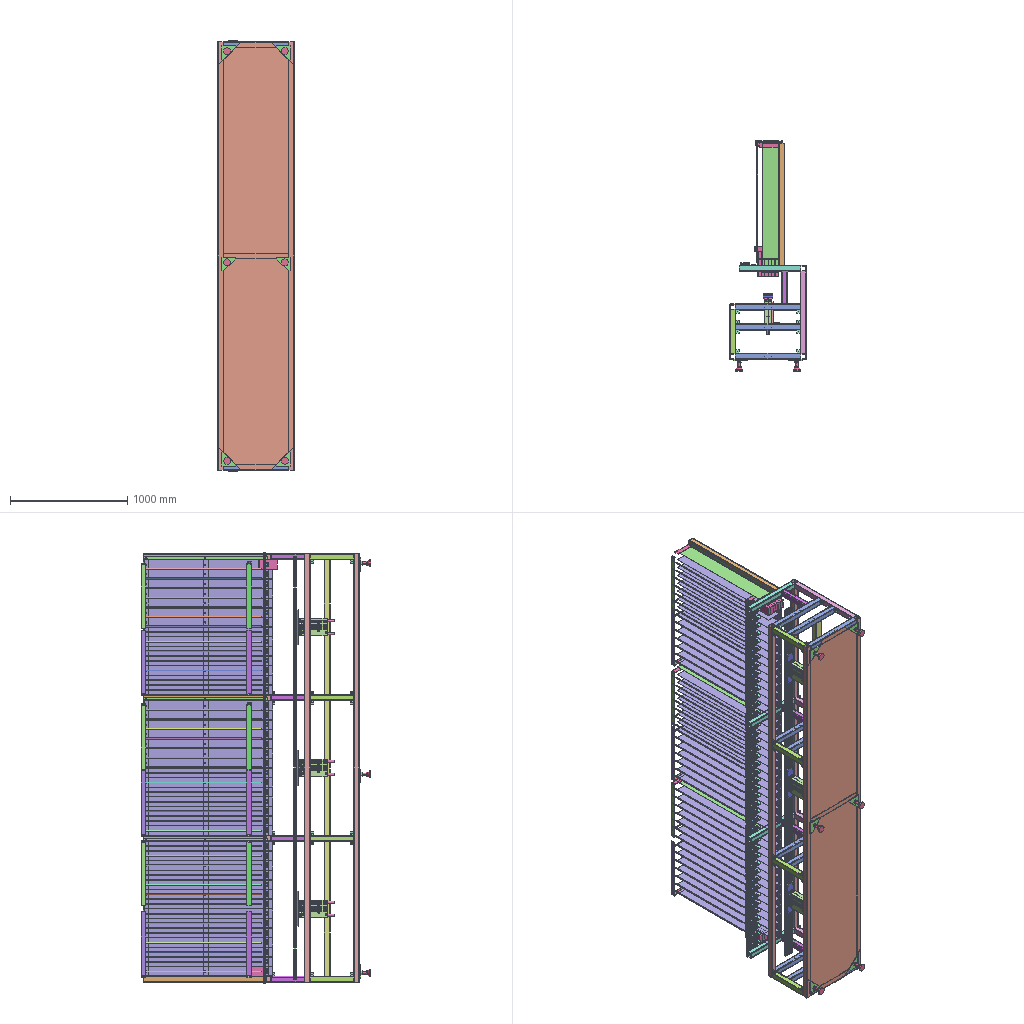Assembly | STEP file | 35 different items | 467 placed | box 650 x 1958 x 3680 mm
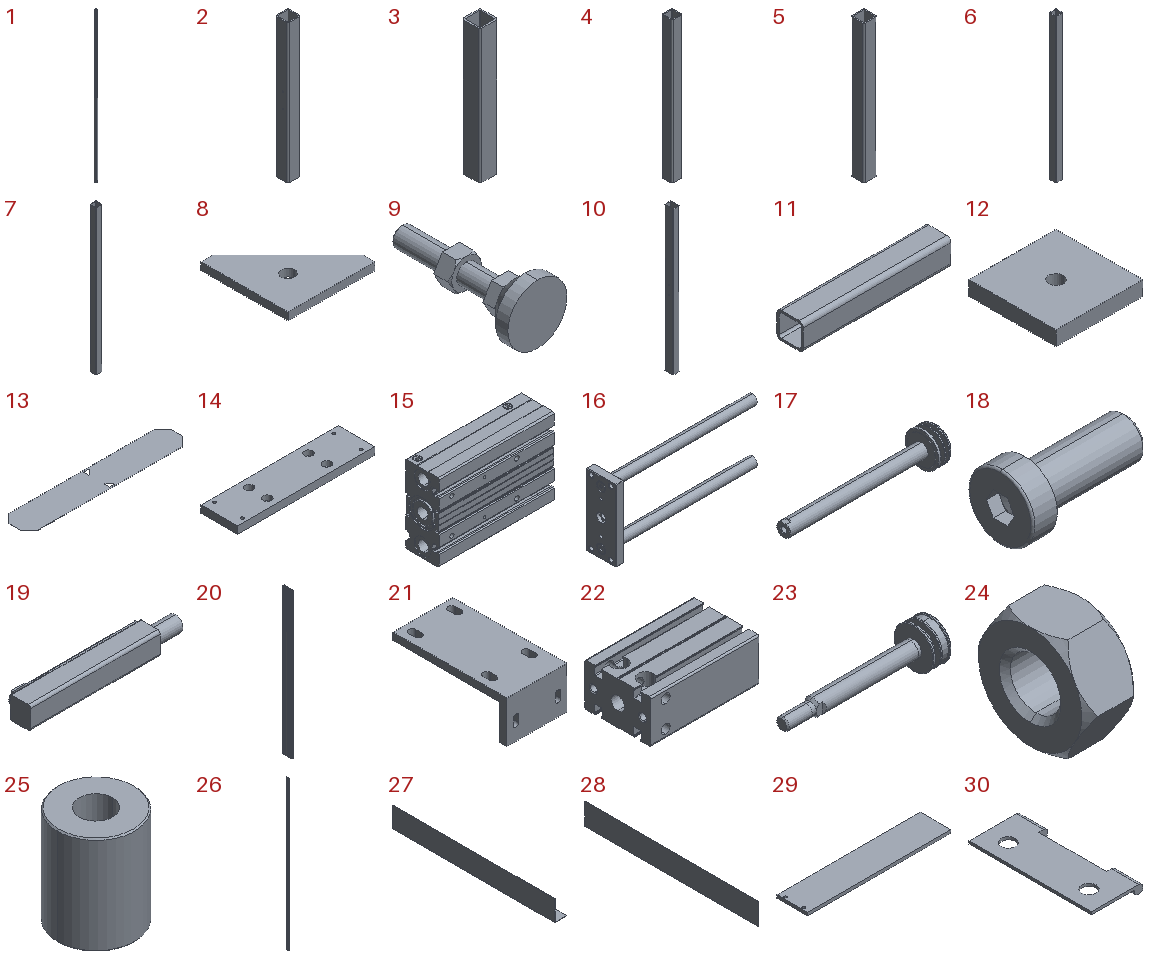Parts list (item | name | quantity | parent item | size | volume):
1 | Square steel 50×50×3650 | x4 | in PN_0007 Battery box frame unit rack | 50 x 50 x 3650 mm | 2611204 mm3
2 | Square steel 50×50×550 | x11 | in PN_0007 Battery box frame unit rack | 50 x 50 x 550 mm | 393155 mm3
3 | Square steel 50×50×370 | x4 | in PN_0007 Battery box frame unit rack | 50 x 50 x 370 mm | 264697 mm3
4 | Square steel 50×50×700 | x4 | in PN_0007 Battery box frame unit rack | 50 x 50 x 700 mm | 500779 mm3
5 | Square steel 50×50×132 | x4 | in PN_0007 Battery box frame unit rack | 50 x 50 x 520 mm | 371896 mm3
6 | Square steel 50×50×1400 | x4 | in PN_0007 Battery box frame unit rack | 50 x 50 x 1040 mm | 744014 mm3
7 | Square steel 50×50×1150 | x9 | in PN_0007 Battery box frame unit rack | 50 x 50 x 1150 mm | 822708 mm3
8 | PN_0001 Adjusting weld plate1 | x6 | in 20APBM adjustable foot pad | 115 x 115 x 10 mm | 79845 mm3
9 | Adjustable foot | x6 | in 20APBM adjustable foot pad | 60 x 138 x 60 mm | 107820 mm3
10 | Square steel 50×70×1150 | x3 | in PN_0007 Battery box frame unit rack | 50 x 70 x 1150 mm | 1005690 mm3
11 | 50X50X280 square tube_default<machined> | x4 | in PN_0007 Battery box frame unit rack | 280 x 50 x 50 mm | 194543 mm3
12 | Small weld block | x32 | in PN_0007 Battery box frame unit rack | 30 x 30 x 5 mm | 4402 mm3
13 | Bottom weld seal plate2 | x1 | in PN_0007 Battery box frame unit rack | 3650 x 650 x 2 mm | 4552100 mm3
14 | PN_0009 connecting plate2 | x3 | in PN_0004 Battery box lift assembly drawing | 300 x 80 x 16 mm | 369093 mm3
15 | TC_L_50x175175_b | x3 | - | 219 x 64 x 148 mm | 1265791 mm3
16 | TC_L_50x175_175fp | x3 | - | 309 x 60 x 146 mm | 316571 mm3
17 | TC_L_50x175_175r | x3 | - | 225 x 49.5 x 49.5 mm | 94503 mm3
18 | - | x3 | - | 31 x 16 x 16 mm | 3053 mm3
19 | CS1_G | x90 | in MD_20x20_S_G_2_MD-20x20-S-G-2 (0) | 30.5 x 5.5 x 4.4 mm | 552.742 mm3
20 | HFS5-2080-1198_HFS5-2080-1380 | x3 | in PN_0004 Battery box lift assembly drawing | 20 x 80 x 1198 mm | 727217 mm3
21 | PN_0002 connecting plate | x3 | in PN_0004 Battery box lift assembly drawing | 100 x 190 x 70 mm | 282725 mm3
22 | - | x42 | in MD_20x20_S_G_2_MD-20x20-S-G-2 (0) | 66 x 40.2 x 26.2 mm | 46950 mm3
23 | - | x42 | in MD_20x20_S_G_2_MD-20x20-S-G-2 (0) | 75 x 19.6 x 19.6 mm | 5220 mm3
24 | - | x42 | in MD_20x20_S_G_2_MD-20x20-S-G-2 (0) | 5 x 11.547 x 10 mm | 329.448 mm3
25 | PN_0003 Press shell nylon post | x42 | in PN_0005 Battery box press-clamp group | 30 x 30 x 38 mm | 22857 mm3
26 | New 20APBM1303-03_HFS5-2080-1380 | x1 | in PN_0005 Battery box press-clamp group | 20 x 80 x 3680 mm | 2231978 mm3
27 | PN_0006 Partition plate | x42 | in 27 | 82 x 1100 x 140 mm | 481847 mm3
28 | PN_0008 Partition plate2 | x3 | in 27 | 30 x 1100 x 140 mm | 365122 mm3
29 | Guard connecting plate | x12 | in Battery guard rail, Mirror battery guard rail | 187 x 40 x 4 mm | 29852 mm3
30 | 1.5 inch micro hinge plate-left | x12 | in 1.5 inch micro hinge plate | 15.15 x 36.2 x 2.5 mm | 425.73 mm3
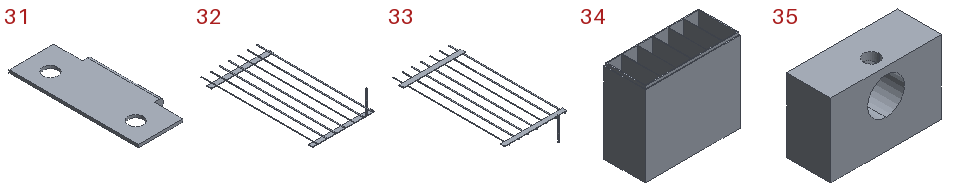31 | 1.5 inch micro hinge plate-right | x12 | in 1.5 inch micro hinge plate | 15.15 x 36.2 x 2.5 mm | 446.218 mm3
32 | Guard baffle | x3 | in Battery guard rail | 550 x 1030 x 211 mm | 463741 mm3
33 | Mirror guard baffle | x3 | in Mirror battery guard rail | 550 x 1030 x 211 mm | 463741 mm3
34 | 20AH housing | x2 | in 27 | 179 x 78 x 157 mm | 325440 mm3
35 | Magnet seat | x6 | in 27 | 30 x 12 x 20 mm | 6542 mm3
Placements (level | parent | child | x y z in mm | rotation matrix by rows), first 355 of 541 lines:
1 | 27 | PN_0007 Battery box frame unit rack | -853.413 -790.459 2150.0 | 1 0 0 0 1 0 0 0 1
2 | PN_0007 Battery box frame unit rack | Square steel 50×50×3650 | -1.422 2.357 1350.0 | 1 0 0 0 1 0 0 0 1
2 | PN_0007 Battery box frame unit rack | Square steel 50×50×3650 | 598.578 2.357 1350.0 | 1 0 0 0 1 0 0 0 1
2 | PN_0007 Battery box frame unit rack | Square steel 50×50×550 | 298.578 2.357 3150.0 | 0 0 -1 0 1 0 1 0 0
2 | PN_0007 Battery box frame unit rack | Square steel 50×50×550 | 298.578 2.357 -450.0 | 0 0 -1 0 1 0 1 0 0
2 | PN_0007 Battery box frame unit rack | Square steel 50×50×370 | -1.422 212.357 3150.0 | 1 0 0 0 0 -1 0 1 0
2 | PN_0007 Battery box frame unit rack | Square steel 50×50×700 | 598.578 377.357 3150.0 | 1 0 0 0 0 -1 0 1 0
2 | PN_0007 Battery box frame unit rack | Square steel 50×50×3650 | -1.422 422.357 1350.0 | 1 0 0 0 1 0 0 0 1
2 | PN_0007 Battery box frame unit rack | Square steel 50×50×700 | 598.578 377.357 1950.0 | 1 0 0 0 0 -1 0 1 0
2 | PN_0007 Battery box frame unit rack | Square steel 50×50×370 | -1.422 212.357 1950.0 | 1 0 0 0 0 -1 0 1 0
2 | PN_0007 Battery box frame unit rack | Square steel 50×50×550 | 298.578 422.357 3150.0 | 0 0 -1 0 1 0 1 0 0
2 | PN_0007 Battery box frame unit rack | Square steel 50×50×550 | 298.578 422.357 1950.0 | 0 0 -1 0 1 0 1 0 0
2 | PN_0007 Battery box frame unit rack | Square steel 50×50×3650 | 598.578 752.357 1350.0 | 1 0 0 0 1 0 0 0 1
2 | PN_0007 Battery box frame unit rack | Square steel 50×50×132 | 313.578 752.357 3150.0 | 0 0 1 0 1 0 -1 0 0
2 | PN_0007 Battery box frame unit rack | Square steel 50×50×132 | 313.578 752.357 1950.0 | 0 0 1 0 1 0 -1 0 0
2 | PN_0007 Battery box frame unit rack | Square steel 50×50×1400 | 416.578 1297.357 3150.0 | 1 0 0 0 0 -1 0 1 -0
2 | PN_0007 Battery box frame unit rack | Square steel 50×50×1400 | 416.578 1297.357 1950.0 | 1 0 0 0 0 -1 0 1 -0
2 | PN_0007 Battery box frame unit rack | Square steel 50×50×1150 | 416.578 1792.357 2550.0 | 1 0 0 0 1 0 0 0 1
2 | PN_0007 Battery box frame unit rack | Square steel 50×50×1150 | 416.578 1282.357 2550.0 | 1 0 0 0 1 0 0 0 1
2 | PN_0007 Battery box frame unit rack | Square steel 50×50×1150 | 416.578 772.357 2550.0 | 1 0 0 0 1 0 0 0 1
2 | PN_0007 Battery box frame unit rack | 20APBM adjustable foot pad | -90.059 -57.18 3070.758 | 0 1 0 0 0 -1 -1 0 0
3 | 20APBM adjustable foot pad | PN_0001 Adjusting weld plate1 | -69.242 98.636 -34.537 | 1 0 0 0 1 0 0 0 1
3 | 20APBM adjustable foot pad | Adjustable foot | -25.242 142.637 63.463 | 1 0 0 0 0 1 0 -1 0
2 | PN_0007 Battery box frame unit rack | 20APBM adjustable foot pad | 519.335 -57.18 3238.637 | -1 0 0 0 0 -1 0 -1 -0
3 | 20APBM adjustable foot pad | PN_0001 Adjusting weld plate1 | -69.242 98.636 -34.537 | 1 0 0 0 1 0 0 0 1
3 | 20APBM adjustable foot pad | Adjustable foot | -25.242 142.637 63.463 | 1 0 0 0 0 1 0 -1 0
2 | PN_0007 Battery box frame unit rack | 20APBM adjustable foot pad | 77.82 -57.18 -538.636 | 1 0 0 0 0 -1 0 1 0
3 | 20APBM adjustable foot pad | PN_0001 Adjusting weld plate1 | -69.242 98.636 -34.537 | 1 0 0 0 1 0 0 0 1
3 | 20APBM adjustable foot pad | Adjustable foot | -25.242 142.637 63.463 | 1 0 0 0 0 1 0 -1 0
2 | PN_0007 Battery box frame unit rack | 20APBM adjustable foot pad | 687.214 -57.18 -370.758 | 0 -1 0 0 0 -1 1 0 0
3 | 20APBM adjustable foot pad | PN_0001 Adjusting weld plate1 | -69.242 98.636 -34.537 | 1 0 0 0 1 0 0 0 1
3 | 20APBM adjustable foot pad | Adjustable foot | -25.242 142.637 63.463 | 1 0 0 0 0 1 0 -1 0
2 | PN_0007 Battery box frame unit rack | Square steel 50×50×132 | 313.578 752.357 750.0 | 0 0 1 0 1 0 -1 0 0
2 | PN_0007 Battery box frame unit rack | Square steel 50×50×132 | 313.578 752.357 -450.0 | 0 0 1 0 1 0 -1 0 0
2 | PN_0007 Battery box frame unit rack | Square steel 50×50×1150 | 416.578 772.357 1350.0 | 1 0 0 0 1 0 0 0 1
2 | PN_0007 Battery box frame unit rack | Square steel 50×50×1150 | 416.578 772.357 150.0 | 1 0 0 0 1 0 0 0 1
2 | PN_0007 Battery box frame unit rack | Square steel 50×50×1400 | 416.578 1297.357 750.0 | 1 0 0 0 0 -1 0 1 -0
2 | PN_0007 Battery box frame unit rack | Square steel 50×50×1400 | 416.578 1297.357 -450.0 | 1 0 0 0 0 -1 0 1 -0
2 | PN_0007 Battery box frame unit rack | Square steel 50×50×700 | 598.578 377.357 750.0 | 1 0 0 0 0 -1 0 1 0
2 | PN_0007 Battery box frame unit rack | Square steel 50×50×700 | 598.578 377.357 -450.0 | 1 0 0 0 0 -1 0 1 0
2 | PN_0007 Battery box frame unit rack | Square steel 50×50×550 | 298.578 422.357 750.0 | 0 0 -1 0 1 0 1 0 0
2 | PN_0007 Battery box frame unit rack | Square steel 50×50×550 | 298.578 422.357 -450.0 | 0 0 -1 0 1 0 1 0 0
2 | PN_0007 Battery box frame unit rack | Square steel 50×50×370 | -1.422 212.357 750.0 | 1 0 0 0 0 -1 0 1 0
2 | PN_0007 Battery box frame unit rack | Square steel 50×50×370 | -1.422 212.357 -450.0 | 1 0 0 0 0 -1 0 1 0
2 | PN_0007 Battery box frame unit rack | Square steel 50×50×1150 | 416.578 1792.357 1350.0 | 1 0 0 0 1 0 0 0 1
2 | PN_0007 Battery box frame unit rack | Square steel 50×50×1150 | 416.578 1792.357 150.0 | 1 0 0 0 1 0 0 0 1
2 | PN_0007 Battery box frame unit rack | Square steel 50×50×1150 | 416.578 1282.357 1350.0 | 1 0 0 0 1 0 0 0 1
2 | PN_0007 Battery box frame unit rack | Square steel 50×50×1150 | 416.578 1282.357 150.0 | 1 0 0 0 1 0 0 0 1
2 | PN_0007 Battery box frame unit rack | Square steel 50×50×550 | 298.578 252.357 3150.0 | 0 0 -1 0 1 0 1 0 0
2 | PN_0007 Battery box frame unit rack | Square steel 50×50×550 | 298.578 252.357 1950.0 | 0 0 -1 0 1 0 1 0 0
2 | PN_0007 Battery box frame unit rack | Square steel 50×50×550 | 298.578 252.357 750.0 | 0 0 -1 0 1 0 1 0 0
2 | PN_0007 Battery box frame unit rack | Square steel 50×50×550 | 298.578 252.357 -450.0 | 0 0 -1 0 1 0 1 0 0
2 | PN_0007 Battery box frame unit rack | Square steel 50×70×1150 | 368.578 252.357 2550.0 | 0 1 0 -1 0 0 0 0 1
2 | PN_0007 Battery box frame unit rack | Square steel 50×70×1150 | 368.578 252.357 1350.0 | 0 1 0 -1 0 0 0 0 1
2 | PN_0007 Battery box frame unit rack | Square steel 50×70×1150 | 368.578 252.357 150.0 | 0 1 0 -1 0 0 0 0 1
2 | PN_0007 Battery box frame unit rack | 20APBM adjustable foot pad | 519.335 -57.18 1438.637 | -1 0 0 0 0 -1 0 -1 -0
3 | 20APBM adjustable foot pad | PN_0001 Adjusting weld plate1 | -69.242 98.636 -34.537 | 1 0 0 0 1 0 0 0 1
3 | 20APBM adjustable foot pad | Adjustable foot | -25.242 142.637 63.463 | 1 0 0 0 0 1 0 -1 0
2 | PN_0007 Battery box frame unit rack | 20APBM adjustable foot pad | -90.059 -57.18 1270.758 | 0 1 0 0 0 -1 -1 0 0
3 | 20APBM adjustable foot pad | PN_0001 Adjusting weld plate1 | -69.242 98.636 -34.537 | 1 0 0 0 1 0 0 0 1
3 | 20APBM adjustable foot pad | Adjustable foot | -25.242 142.637 63.463 | 1 0 0 0 0 1 0 -1 0
2 | PN_0007 Battery box frame unit rack | Square steel 50×50×550 | 298.578 2.357 1350.0 | 0 0 -1 0 1 0 1 0 0
2 | PN_0007 Battery box frame unit rack | 50X50X280 square tube_default<machined> | 441.578 587.357 3150.0 | 0 1 0 -1 0 0 0 0 1
2 | PN_0007 Battery box frame unit rack | 50X50X280 square tube_default<machined> | 441.578 587.357 1950.0 | 0 1 0 -1 0 0 0 0 1
2 | PN_0007 Battery box frame unit rack | 50X50X280 square tube_default<machined> | 441.578 587.357 750.0 | 0 1 0 -1 0 0 0 0 1
2 | PN_0007 Battery box frame unit rack | 50X50X280 square tube_default<machined> | 441.578 587.357 -450.0 | 0 1 0 -1 0 0 0 0 1
2 | PN_0007 Battery box frame unit rack | Small weld block | -13.922 382.357 -410.0 | 0 0 -1 0 -1 0 -1 0 -0
2 | PN_0007 Battery box frame unit rack | Small weld block | -13.922 42.357 -410.0 | 0 0 -1 0 -1 0 -1 0 -0
2 | PN_0007 Battery box frame unit rack | Small weld block | -13.922 382.357 710.0 | 0 0 -1 0 -1 0 -1 0 -0
2 | PN_0007 Battery box frame unit rack | Small weld block | -13.922 42.357 710.0 | 0 0 -1 0 -1 0 -1 0 -0
2 | PN_0007 Battery box frame unit rack | Small weld block | -13.922 382.357 1910.0 | 0 0 -1 0 -1 0 -1 0 -0
2 | PN_0007 Battery box frame unit rack | Small weld block | -13.922 382.357 3110.0 | 0 0 -1 0 -1 0 -1 0 -0
2 | PN_0007 Battery box frame unit rack | Small weld block | -13.922 42.357 790.0 | 0 0 -1 0 -1 0 -1 0 -0
2 | PN_0007 Battery box frame unit rack | Small weld block | -13.922 42.357 1990.0 | 0 0 -1 0 -1 0 -1 0 -0
2 | PN_0007 Battery box frame unit rack | Small weld block | -13.922 382.357 790.0 | 0 0 -1 0 -1 0 -1 0 -0
2 | PN_0007 Battery box frame unit rack | Small weld block | -13.922 382.357 1990.0 | 0 0 -1 0 -1 0 -1 0 -0
2 | PN_0007 Battery box frame unit rack | Small weld block | -13.922 42.357 1910.0 | 0 0 -1 0 -1 0 -1 0 -0
2 | PN_0007 Battery box frame unit rack | Small weld block | -13.922 42.357 3110.0 | 0 0 -1 0 -1 0 -1 0 -0
2 | PN_0007 Battery box frame unit rack | Small weld block | 611.078 42.357 -410.0 | 0 0 -1 0 -1 0 -1 0 -0
2 | PN_0007 Battery box frame unit rack | Small weld block | 611.078 712.357 -410.0 | 0 0 -1 0 -1 0 -1 0 -0
2 | PN_0007 Battery box frame unit rack | Small weld block | 611.078 712.357 710.0 | 0 0 1 0 -1 0 1 0 0
2 | PN_0007 Battery box frame unit rack | Small weld block | 611.078 42.357 710.0 | 0 0 1 0 -1 0 1 0 0
2 | PN_0007 Battery box frame unit rack | Small weld block | 611.078 712.357 790.0 | 0 0 -1 0 -1 0 -1 0 -0
2 | PN_0007 Battery box frame unit rack | Small weld block | 611.078 712.357 1990.0 | 0 0 -1 0 -1 0 -1 0 -0
2 | PN_0007 Battery box frame unit rack | Small weld block | 611.078 42.357 790.0 | 0 0 -1 0 -1 0 -1 0 -0
2 | PN_0007 Battery box frame unit rack | Small weld block | 611.078 42.357 1990.0 | 0 0 -1 0 -1 0 -1 0 -0
2 | PN_0007 Battery box frame unit rack | Small weld block | 611.078 42.357 1910.0 | 0 0 1 0 -1 0 1 0 0
2 | PN_0007 Battery box frame unit rack | Small weld block | 611.078 42.357 3110.0 | 0 0 1 0 -1 0 1 0 0
2 | PN_0007 Battery box frame unit rack | Small weld block | 611.078 712.357 1910.0 | 0 0 1 0 -1 0 1 0 0
2 | PN_0007 Battery box frame unit rack | Small weld block | 611.078 712.357 3110.0 | 0 0 1 0 -1 0 1 0 0
2 | PN_0007 Battery box frame unit rack | Small weld block | 38.578 382.357 3162.5 | -1 0 0 0 -1 0 0 0 1
2 | PN_0007 Battery box frame unit rack | Small weld block | 38.578 292.357 3162.5 | -1 0 0 0 -1 0 0 0 1
2 | PN_0007 Battery box frame unit rack | Small weld block | 38.578 212.357 3162.5 | -1 0 0 0 -1 0 0 0 1
2 | PN_0007 Battery box frame unit rack | Small weld block | 38.578 42.357 3162.5 | -1 0 0 0 -1 0 0 0 1
2 | PN_0007 Battery box frame unit rack | Small weld block | 558.578 382.357 3162.5 | 1 0 0 0 -1 0 0 0 -1
2 | PN_0007 Battery box frame unit rack | Small weld block | 558.578 292.357 3162.5 | 1 0 0 0 -1 0 0 0 -1
2 | PN_0007 Battery box frame unit rack | Small weld block | 558.578 212.357 3162.5 | 1 0 0 0 -1 0 0 0 -1
2 | PN_0007 Battery box frame unit rack | Small weld block | 558.578 42.357 3162.5 | 1 0 0 0 -1 0 0 0 -1
2 | PN_0007 Battery box frame unit rack | Bottom weld seal plate2 | 298.578 -22.643 3150.0 | 0 1 0 0 0 -1 -1 0 -0
1 | 27 | PN_0004 Battery box lift assembly drawing | -522.835 -513.102 4700.0 | 0 0 1 0 1 0 -1 0 0
2 | PN_0004 Battery box lift assembly drawing | PN_0009 connecting plate2 | -0.0 222.0 -32.0 | 1 0 0 0 0 1 0 -1 0
2 | PN_0004 Battery box lift assembly drawing | subassembly 2 | -0.0 194.0 -32.0 | 0 -1 0 -1 0 0 0 0 -1
3 | subassembly 2 | TC_L_50x175175_b | 0.0 0.0 0.0 | 1 0 0 0 0 -1 0 1 0
3 | subassembly 2 | TC_L_50x175_175fp | -28.0 -0.0 -0.0 | 1 0 0 0 0 -1 0 1 0
3 | subassembly 2 | TC_L_50x175_175r | -12.0 -0.0 -0.0 | 1 0 0 0 1 0 0 0 1
3 | subassembly 2 | subassembly 3 | -22.0 -0.0 -0.0 | 1 0 0 0 0 -1 0 1 0
3 | subassembly 2 | CS1_G | 1.0 16.6 24.5 | 1 0 0 0 0 -1 0 1 0
3 | subassembly 2 | CS1_G | 218.0 -16.6 -24.5 | -1 0 0 0 0 -1 0 -1 0
2 | PN_0004 Battery box lift assembly drawing | HFS5-2080-1198_HFS5-2080-1380 | -0.0 248.0 -32.0 | 0 0 -1 -1 0 0 0 1 0
2 | PN_0004 Battery box lift assembly drawing | PN_0002 connecting plate | -0.0 -0.0 -0.0 | -1 0 0 0 1 0 0 0 -1
1 | 27 | PN_0004 Battery box lift assembly drawing | -522.835 -513.102 3500.0 | 0 0 1 0 1 0 -1 0 0
2 | PN_0004 Battery box lift assembly drawing | PN_0009 connecting plate2 | -0.0 222.0 -32.0 | 1 0 0 0 0 1 0 -1 0
2 | PN_0004 Battery box lift assembly drawing | subassembly 2 | -0.0 194.0 -32.0 | 0 -1 0 -1 0 0 0 0 -1
3 | subassembly 2 | TC_L_50x175175_b | 0.0 0.0 0.0 | 1 0 0 0 0 -1 0 1 0
3 | subassembly 2 | TC_L_50x175_175fp | -28.0 -0.0 -0.0 | 1 0 0 0 0 -1 0 1 0
3 | subassembly 2 | TC_L_50x175_175r | -12.0 -0.0 -0.0 | 1 0 0 0 1 0 0 0 1
3 | subassembly 2 | subassembly 3 | -22.0 -0.0 -0.0 | 1 0 0 0 0 -1 0 1 0
3 | subassembly 2 | CS1_G | 1.0 16.6 24.5 | 1 0 0 0 0 -1 0 1 0
3 | subassembly 2 | CS1_G | 218.0 -16.6 -24.5 | -1 0 0 0 0 -1 0 -1 0
2 | PN_0004 Battery box lift assembly drawing | HFS5-2080-1198_HFS5-2080-1380 | -0.0 248.0 -32.0 | 0 0 -1 -1 0 0 0 1 0
2 | PN_0004 Battery box lift assembly drawing | PN_0002 connecting plate | -0.0 -0.0 -0.0 | -1 0 0 0 1 0 0 0 -1
1 | 27 | PN_0004 Battery box lift assembly drawing | -522.835 -513.102 2300.0 | 0 0 1 0 1 0 -1 0 0
2 | PN_0004 Battery box lift assembly drawing | PN_0009 connecting plate2 | -0.0 222.0 -32.0 | 1 0 0 0 0 1 0 -1 0
2 | PN_0004 Battery box lift assembly drawing | subassembly 2 | -0.0 194.0 -32.0 | 0 -1 0 -1 0 0 0 0 -1
3 | subassembly 2 | TC_L_50x175175_b | 0.0 0.0 0.0 | 1 0 0 0 0 -1 0 1 0
3 | subassembly 2 | TC_L_50x175_175fp | -28.0 -0.0 -0.0 | 1 0 0 0 0 -1 0 1 0
3 | subassembly 2 | TC_L_50x175_175r | -12.0 -0.0 -0.0 | 1 0 0 0 1 0 0 0 1
3 | subassembly 2 | subassembly 3 | -22.0 -0.0 -0.0 | 1 0 0 0 0 -1 0 1 0
3 | subassembly 2 | CS1_G | 1.0 16.6 24.5 | 1 0 0 0 0 -1 0 1 0
3 | subassembly 2 | CS1_G | 218.0 -16.6 -24.5 | -1 0 0 0 0 -1 0 -1 0
2 | PN_0004 Battery box lift assembly drawing | HFS5-2080-1198_HFS5-2080-1380 | -0.0 248.0 -32.0 | 0 0 -1 -1 0 0 0 1 0
2 | PN_0004 Battery box lift assembly drawing | PN_0002 connecting plate | -0.0 -0.0 -0.0 | -1 0 0 0 1 0 0 0 -1
1 | 27 | PN_0005 Battery box press-clamp group | -602.881 -25.18 1667.5 | -1 0 0 0 1 0 0 0 -1
2 | PN_0005 Battery box press-clamp group | MD_20x20_S_G_2_MD-20x20-S-G-2 (0) | 109.954 -0.8216 -3567.4 | 1 0 0 0 0 1 0 -1 0
3 | MD_20x20_S_G_2_MD-20x20-S-G-2 (0) | subassembly 4 | -0.0 -0.0 -0.0 | 1 0 0 0 1 0 0 0 1
3 | MD_20x20_S_G_2_MD-20x20-S-G-2 (0) | subassembly 5 | -0.0 -0.0 -0.0 | 1 0 0 0 0 -1 0 1 0
3 | MD_20x20_S_G_2_MD-20x20-S-G-2 (0) | subassembly 6 | -9.0 -0.0 -0.0 | -1 0 0 0 0 -1 0 -1 0
3 | MD_20x20_S_G_2_MD-20x20-S-G-2 (0) | CS1_G | 14.65 12.0 7.5 | 1 0 0 0 0 -1 0 1 0
3 | MD_20x20_S_G_2_MD-20x20-S-G-2 (0) | CS1_G | 65.0 -12.0 -7.5 | -1 0 0 0 0 -1 0 -1 0
2 | PN_0005 Battery box press-clamp group | MD_20x20_S_G_2_MD-20x20-S-G-2 (0) | 109.954 -0.8216 -3485.4 | 1 0 0 0 0 1 0 -1 0
3 | MD_20x20_S_G_2_MD-20x20-S-G-2 (0) | subassembly 4 | -0.0 -0.0 -0.0 | 1 0 0 0 1 0 0 0 1
3 | MD_20x20_S_G_2_MD-20x20-S-G-2 (0) | subassembly 5 | -0.0 -0.0 -0.0 | 1 0 0 0 0 -1 0 1 0
3 | MD_20x20_S_G_2_MD-20x20-S-G-2 (0) | subassembly 6 | -9.0 -0.0 -0.0 | -1 0 0 0 0 -1 0 -1 0
3 | MD_20x20_S_G_2_MD-20x20-S-G-2 (0) | CS1_G | 14.65 12.0 7.5 | 1 0 0 0 0 -1 0 1 0
3 | MD_20x20_S_G_2_MD-20x20-S-G-2 (0) | CS1_G | 65.0 -12.0 -7.5 | -1 0 0 0 0 -1 0 -1 0
2 | PN_0005 Battery box press-clamp group | MD_20x20_S_G_2_MD-20x20-S-G-2 (0) | 109.954 -0.8216 -3403.4 | 1 0 0 0 0 1 0 -1 0
3 | MD_20x20_S_G_2_MD-20x20-S-G-2 (0) | subassembly 4 | -0.0 -0.0 -0.0 | 1 0 0 0 1 0 0 0 1
3 | MD_20x20_S_G_2_MD-20x20-S-G-2 (0) | subassembly 5 | -0.0 -0.0 -0.0 | 1 0 0 0 0 -1 0 1 0
3 | MD_20x20_S_G_2_MD-20x20-S-G-2 (0) | subassembly 6 | -9.0 -0.0 -0.0 | -1 0 0 0 0 -1 0 -1 0
3 | MD_20x20_S_G_2_MD-20x20-S-G-2 (0) | CS1_G | 14.65 12.0 7.5 | 1 0 0 0 0 -1 0 1 0
3 | MD_20x20_S_G_2_MD-20x20-S-G-2 (0) | CS1_G | 65.0 -12.0 -7.5 | -1 0 0 0 0 -1 0 -1 0
2 | PN_0005 Battery box press-clamp group | MD_20x20_S_G_2_MD-20x20-S-G-2 (0) | 109.954 -0.8216 -3321.4 | 1 0 0 0 0 1 0 -1 0
3 | MD_20x20_S_G_2_MD-20x20-S-G-2 (0) | subassembly 4 | -0.0 -0.0 -0.0 | 1 0 0 0 1 0 0 0 1
3 | MD_20x20_S_G_2_MD-20x20-S-G-2 (0) | subassembly 5 | -0.0 -0.0 -0.0 | 1 0 0 0 0 -1 0 1 0
3 | MD_20x20_S_G_2_MD-20x20-S-G-2 (0) | subassembly 6 | -9.0 -0.0 -0.0 | -1 0 0 0 0 -1 0 -1 0
3 | MD_20x20_S_G_2_MD-20x20-S-G-2 (0) | CS1_G | 14.65 12.0 7.5 | 1 0 0 0 0 -1 0 1 0
3 | MD_20x20_S_G_2_MD-20x20-S-G-2 (0) | CS1_G | 65.0 -12.0 -7.5 | -1 0 0 0 0 -1 0 -1 0
2 | PN_0005 Battery box press-clamp group | MD_20x20_S_G_2_MD-20x20-S-G-2 (0) | 109.954 -0.8216 -3239.4 | 1 0 0 0 0 1 0 -1 0
3 | MD_20x20_S_G_2_MD-20x20-S-G-2 (0) | subassembly 4 | -0.0 -0.0 -0.0 | 1 0 0 0 1 0 0 0 1
3 | MD_20x20_S_G_2_MD-20x20-S-G-2 (0) | subassembly 5 | -0.0 -0.0 -0.0 | 1 0 0 0 0 -1 0 1 0
3 | MD_20x20_S_G_2_MD-20x20-S-G-2 (0) | subassembly 6 | -9.0 -0.0 -0.0 | -1 0 0 0 0 -1 0 -1 0
3 | MD_20x20_S_G_2_MD-20x20-S-G-2 (0) | CS1_G | 14.65 12.0 7.5 | 1 0 0 0 0 -1 0 1 0
3 | MD_20x20_S_G_2_MD-20x20-S-G-2 (0) | CS1_G | 65.0 -12.0 -7.5 | -1 0 0 0 0 -1 0 -1 0
2 | PN_0005 Battery box press-clamp group | MD_20x20_S_G_2_MD-20x20-S-G-2 (0) | 109.954 -0.8216 -3157.4 | 1 0 0 0 0 1 0 -1 0
3 | MD_20x20_S_G_2_MD-20x20-S-G-2 (0) | subassembly 4 | -0.0 -0.0 -0.0 | 1 0 0 0 1 0 0 0 1
3 | MD_20x20_S_G_2_MD-20x20-S-G-2 (0) | subassembly 5 | -0.0 -0.0 -0.0 | 1 0 0 0 0 -1 0 1 0
3 | MD_20x20_S_G_2_MD-20x20-S-G-2 (0) | subassembly 6 | -9.0 -0.0 -0.0 | -1 0 0 0 0 -1 0 -1 0
3 | MD_20x20_S_G_2_MD-20x20-S-G-2 (0) | CS1_G | 14.65 12.0 7.5 | 1 0 0 0 0 -1 0 1 0
3 | MD_20x20_S_G_2_MD-20x20-S-G-2 (0) | CS1_G | 65.0 -12.0 -7.5 | -1 0 0 0 0 -1 0 -1 0
2 | PN_0005 Battery box press-clamp group | MD_20x20_S_G_2_MD-20x20-S-G-2 (0) | 109.954 -0.8216 -3075.4 | 1 0 0 0 0 1 0 -1 0
3 | MD_20x20_S_G_2_MD-20x20-S-G-2 (0) | subassembly 4 | -0.0 -0.0 -0.0 | 1 0 0 0 1 0 0 0 1
3 | MD_20x20_S_G_2_MD-20x20-S-G-2 (0) | subassembly 5 | -0.0 -0.0 -0.0 | 1 0 0 0 0 -1 0 1 0
3 | MD_20x20_S_G_2_MD-20x20-S-G-2 (0) | subassembly 6 | -9.0 -0.0 -0.0 | -1 0 0 0 0 -1 0 -1 0
3 | MD_20x20_S_G_2_MD-20x20-S-G-2 (0) | CS1_G | 14.65 12.0 7.5 | 1 0 0 0 0 -1 0 1 0
3 | MD_20x20_S_G_2_MD-20x20-S-G-2 (0) | CS1_G | 65.0 -12.0 -7.5 | -1 0 0 0 0 -1 0 -1 0
2 | PN_0005 Battery box press-clamp group | MD_20x20_S_G_2_MD-20x20-S-G-2 (0) | 109.954 -0.8216 -2993.4 | 1 0 0 0 0 1 0 -1 0
3 | MD_20x20_S_G_2_MD-20x20-S-G-2 (0) | subassembly 4 | -0.0 -0.0 -0.0 | 1 0 0 0 1 0 0 0 1
3 | MD_20x20_S_G_2_MD-20x20-S-G-2 (0) | subassembly 5 | -0.0 -0.0 -0.0 | 1 0 0 0 0 -1 0 1 0
3 | MD_20x20_S_G_2_MD-20x20-S-G-2 (0) | subassembly 6 | -9.0 -0.0 -0.0 | -1 0 0 0 0 -1 0 -1 0
3 | MD_20x20_S_G_2_MD-20x20-S-G-2 (0) | CS1_G | 14.65 12.0 7.5 | 1 0 0 0 0 -1 0 1 0
3 | MD_20x20_S_G_2_MD-20x20-S-G-2 (0) | CS1_G | 65.0 -12.0 -7.5 | -1 0 0 0 0 -1 0 -1 0
2 | PN_0005 Battery box press-clamp group | MD_20x20_S_G_2_MD-20x20-S-G-2 (0) | 109.954 -0.8216 -2911.4 | 1 0 0 0 0 1 0 -1 0
3 | MD_20x20_S_G_2_MD-20x20-S-G-2 (0) | subassembly 4 | -0.0 -0.0 -0.0 | 1 0 0 0 1 0 0 0 1
3 | MD_20x20_S_G_2_MD-20x20-S-G-2 (0) | subassembly 5 | -0.0 -0.0 -0.0 | 1 0 0 0 0 -1 0 1 0
3 | MD_20x20_S_G_2_MD-20x20-S-G-2 (0) | subassembly 6 | -9.0 -0.0 -0.0 | -1 0 0 0 0 -1 0 -1 0
3 | MD_20x20_S_G_2_MD-20x20-S-G-2 (0) | CS1_G | 14.65 12.0 7.5 | 1 0 0 0 0 -1 0 1 0
3 | MD_20x20_S_G_2_MD-20x20-S-G-2 (0) | CS1_G | 65.0 -12.0 -7.5 | -1 0 0 0 0 -1 0 -1 0
2 | PN_0005 Battery box press-clamp group | MD_20x20_S_G_2_MD-20x20-S-G-2 (0) | 109.954 -0.8216 -2829.4 | 1 0 0 0 0 1 0 -1 0
3 | MD_20x20_S_G_2_MD-20x20-S-G-2 (0) | subassembly 4 | -0.0 -0.0 -0.0 | 1 0 0 0 1 0 0 0 1
3 | MD_20x20_S_G_2_MD-20x20-S-G-2 (0) | subassembly 5 | -0.0 -0.0 -0.0 | 1 0 0 0 0 -1 0 1 0
3 | MD_20x20_S_G_2_MD-20x20-S-G-2 (0) | subassembly 6 | -9.0 -0.0 -0.0 | -1 0 0 0 0 -1 0 -1 0
3 | MD_20x20_S_G_2_MD-20x20-S-G-2 (0) | CS1_G | 14.65 12.0 7.5 | 1 0 0 0 0 -1 0 1 0
3 | MD_20x20_S_G_2_MD-20x20-S-G-2 (0) | CS1_G | 65.0 -12.0 -7.5 | -1 0 0 0 0 -1 0 -1 0
2 | PN_0005 Battery box press-clamp group | MD_20x20_S_G_2_MD-20x20-S-G-2 (0) | 109.954 -0.8216 -2747.4 | 1 0 0 0 0 1 0 -1 0
3 | MD_20x20_S_G_2_MD-20x20-S-G-2 (0) | subassembly 4 | -0.0 -0.0 -0.0 | 1 0 0 0 1 0 0 0 1
3 | MD_20x20_S_G_2_MD-20x20-S-G-2 (0) | subassembly 5 | -0.0 -0.0 -0.0 | 1 0 0 0 0 -1 0 1 0
3 | MD_20x20_S_G_2_MD-20x20-S-G-2 (0) | subassembly 6 | -9.0 -0.0 -0.0 | -1 0 0 0 0 -1 0 -1 0
3 | MD_20x20_S_G_2_MD-20x20-S-G-2 (0) | CS1_G | 14.65 12.0 7.5 | 1 0 0 0 0 -1 0 1 0
3 | MD_20x20_S_G_2_MD-20x20-S-G-2 (0) | CS1_G | 65.0 -12.0 -7.5 | -1 0 0 0 0 -1 0 -1 0
2 | PN_0005 Battery box press-clamp group | MD_20x20_S_G_2_MD-20x20-S-G-2 (0) | 109.954 -0.8216 -2665.4 | 1 0 0 0 0 1 0 -1 0
3 | MD_20x20_S_G_2_MD-20x20-S-G-2 (0) | subassembly 4 | -0.0 -0.0 -0.0 | 1 0 0 0 1 0 0 0 1
3 | MD_20x20_S_G_2_MD-20x20-S-G-2 (0) | subassembly 5 | -0.0 -0.0 -0.0 | 1 0 0 0 0 -1 0 1 0
3 | MD_20x20_S_G_2_MD-20x20-S-G-2 (0) | subassembly 6 | -9.0 -0.0 -0.0 | -1 0 0 0 0 -1 0 -1 0
3 | MD_20x20_S_G_2_MD-20x20-S-G-2 (0) | CS1_G | 14.65 12.0 7.5 | 1 0 0 0 0 -1 0 1 0
3 | MD_20x20_S_G_2_MD-20x20-S-G-2 (0) | CS1_G | 65.0 -12.0 -7.5 | -1 0 0 0 0 -1 0 -1 0
2 | PN_0005 Battery box press-clamp group | MD_20x20_S_G_2_MD-20x20-S-G-2 (0) | 109.954 -0.8216 -2583.4 | 1 0 0 0 0 1 0 -1 0
3 | MD_20x20_S_G_2_MD-20x20-S-G-2 (0) | subassembly 4 | -0.0 -0.0 -0.0 | 1 0 0 0 1 0 0 0 1
3 | MD_20x20_S_G_2_MD-20x20-S-G-2 (0) | subassembly 5 | -0.0 -0.0 -0.0 | 1 0 0 0 0 -1 0 1 0
3 | MD_20x20_S_G_2_MD-20x20-S-G-2 (0) | subassembly 6 | -9.0 -0.0 -0.0 | -1 0 0 0 0 -1 0 -1 0
3 | MD_20x20_S_G_2_MD-20x20-S-G-2 (0) | CS1_G | 14.65 12.0 7.5 | 1 0 0 0 0 -1 0 1 0
3 | MD_20x20_S_G_2_MD-20x20-S-G-2 (0) | CS1_G | 65.0 -12.0 -7.5 | -1 0 0 0 0 -1 0 -1 0
2 | PN_0005 Battery box press-clamp group | MD_20x20_S_G_2_MD-20x20-S-G-2 (0) | 109.954 -0.8216 -2501.4 | 1 0 0 0 0 1 0 -1 0
3 | MD_20x20_S_G_2_MD-20x20-S-G-2 (0) | subassembly 4 | -0.0 -0.0 -0.0 | 1 0 0 0 1 0 0 0 1
3 | MD_20x20_S_G_2_MD-20x20-S-G-2 (0) | subassembly 5 | -0.0 -0.0 -0.0 | 1 0 0 0 0 -1 0 1 0
3 | MD_20x20_S_G_2_MD-20x20-S-G-2 (0) | subassembly 6 | -9.0 -0.0 -0.0 | -1 0 0 0 0 -1 0 -1 0
3 | MD_20x20_S_G_2_MD-20x20-S-G-2 (0) | CS1_G | 14.65 12.0 7.5 | 1 0 0 0 0 -1 0 1 0
3 | MD_20x20_S_G_2_MD-20x20-S-G-2 (0) | CS1_G | 65.0 -12.0 -7.5 | -1 0 0 0 0 -1 0 -1 0
2 | PN_0005 Battery box press-clamp group | PN_0003 Press shell nylon post | 76.954 -0.8216 -3567.4 | 0 0 -1 0.9341 -0.3571 0 -0.3571 -0.9341 -0
2 | PN_0005 Battery box press-clamp group | PN_0003 Press shell nylon post | 76.954 -0.8216 -3485.4 | 0 0 -1 0.9341 -0.3571 0 -0.3571 -0.9341 -0
2 | PN_0005 Battery box press-clamp group | PN_0003 Press shell nylon post | 76.954 -0.8216 -3403.4 | 0 0 -1 0.9341 -0.3571 0 -0.3571 -0.9341 -0
2 | PN_0005 Battery box press-clamp group | PN_0003 Press shell nylon post | 76.954 -0.8216 -3321.4 | 0 0 -1 0.9341 -0.3571 0 -0.3571 -0.9341 -0
2 | PN_0005 Battery box press-clamp group | PN_0003 Press shell nylon post | 76.954 -0.8216 -3239.4 | 0 0 -1 0.9341 -0.3571 0 -0.3571 -0.9341 -0
2 | PN_0005 Battery box press-clamp group | PN_0003 Press shell nylon post | 76.954 -0.8216 -3157.4 | 0 0 -1 0.9341 -0.3571 0 -0.3571 -0.9341 -0
2 | PN_0005 Battery box press-clamp group | PN_0003 Press shell nylon post | 76.954 -0.8216 -3075.4 | 0 0 -1 0.9341 -0.3571 0 -0.3571 -0.9341 -0
2 | PN_0005 Battery box press-clamp group | PN_0003 Press shell nylon post | 76.954 -0.8216 -2993.4 | 0 0 -1 0.9341 -0.3571 0 -0.3571 -0.9341 -0
2 | PN_0005 Battery box press-clamp group | PN_0003 Press shell nylon post | 76.954 -0.8216 -2911.4 | 0 0 -1 0.9341 -0.3571 0 -0.3571 -0.9341 -0
2 | PN_0005 Battery box press-clamp group | PN_0003 Press shell nylon post | 76.954 -0.8216 -2829.4 | 0 0 -1 0.9341 -0.3571 0 -0.3571 -0.9341 -0
2 | PN_0005 Battery box press-clamp group | PN_0003 Press shell nylon post | 76.954 -0.8216 -2747.4 | 0 0 -1 0.9341 -0.3571 0 -0.3571 -0.9341 -0
2 | PN_0005 Battery box press-clamp group | PN_0003 Press shell nylon post | 76.954 -0.8216 -2665.4 | 0 0 -1 0.9341 -0.3571 0 -0.3571 -0.9341 -0
2 | PN_0005 Battery box press-clamp group | PN_0003 Press shell nylon post | 76.954 -0.8216 -2583.4 | 0 0 -1 0.9341 -0.3571 0 -0.3571 -0.9341 -0
2 | PN_0005 Battery box press-clamp group | PN_0003 Press shell nylon post | 76.954 -0.8216 -2501.4 | 0 0 -1 0.9341 -0.3571 0 -0.3571 -0.9341 -0
2 | PN_0005 Battery box press-clamp group | New 20APBM1303-03_HFS5-2080-1380 | 148.954 22.078 7.5 | 0 -1 0 1 0 0 0 0 1
2 | PN_0005 Battery box press-clamp group | MD_20x20_S_G_2_MD-20x20-S-G-2 (0) | 109.954 -0.8216 -2367.4 | 1 0 0 0 0 1 0 -1 0
3 | MD_20x20_S_G_2_MD-20x20-S-G-2 (0) | subassembly 4 | -0.0 -0.0 -0.0 | 1 0 0 0 1 0 0 0 1
3 | MD_20x20_S_G_2_MD-20x20-S-G-2 (0) | subassembly 5 | -0.0 -0.0 -0.0 | 1 0 0 0 0 -1 0 1 0
3 | MD_20x20_S_G_2_MD-20x20-S-G-2 (0) | subassembly 6 | -9.0 -0.0 -0.0 | -1 0 0 0 0 -1 0 -1 0
3 | MD_20x20_S_G_2_MD-20x20-S-G-2 (0) | CS1_G | 14.65 12.0 7.5 | 1 0 0 0 0 -1 0 1 0
3 | MD_20x20_S_G_2_MD-20x20-S-G-2 (0) | CS1_G | 65.0 -12.0 -7.5 | -1 0 0 0 0 -1 0 -1 0
2 | PN_0005 Battery box press-clamp group | MD_20x20_S_G_2_MD-20x20-S-G-2 (0) | 109.954 -0.8216 -1167.4 | 1 0 0 0 0 1 0 -1 0
3 | MD_20x20_S_G_2_MD-20x20-S-G-2 (0) | subassembly 4 | -0.0 -0.0 -0.0 | 1 0 0 0 1 0 0 0 1
3 | MD_20x20_S_G_2_MD-20x20-S-G-2 (0) | subassembly 5 | -0.0 -0.0 -0.0 | 1 0 0 0 0 -1 0 1 0
3 | MD_20x20_S_G_2_MD-20x20-S-G-2 (0) | subassembly 6 | -9.0 -0.0 -0.0 | -1 0 0 0 0 -1 0 -1 0
3 | MD_20x20_S_G_2_MD-20x20-S-G-2 (0) | CS1_G | 14.65 12.0 7.5 | 1 0 0 0 0 -1 0 1 0
3 | MD_20x20_S_G_2_MD-20x20-S-G-2 (0) | CS1_G | 65.0 -12.0 -7.5 | -1 0 0 0 0 -1 0 -1 0
2 | PN_0005 Battery box press-clamp group | PN_0003 Press shell nylon post | 76.954 -0.8216 -2367.4 | 0 0 -1 0.9341 -0.3571 0 -0.3571 -0.9341 -0
2 | PN_0005 Battery box press-clamp group | PN_0003 Press shell nylon post | 76.954 -0.8216 -1167.4 | 0 0 -1 0.9341 -0.3571 0 -0.3571 -0.9341 -0
2 | PN_0005 Battery box press-clamp group | MD_20x20_S_G_2_MD-20x20-S-G-2 (0) | 109.954 -0.8216 -2285.4 | 1 0 0 0 0 1 0 -1 0
3 | MD_20x20_S_G_2_MD-20x20-S-G-2 (0) | subassembly 4 | -0.0 -0.0 -0.0 | 1 0 0 0 1 0 0 0 1
3 | MD_20x20_S_G_2_MD-20x20-S-G-2 (0) | subassembly 5 | -0.0 -0.0 -0.0 | 1 0 0 0 0 -1 0 1 0
3 | MD_20x20_S_G_2_MD-20x20-S-G-2 (0) | subassembly 6 | -9.0 -0.0 -0.0 | -1 0 0 0 0 -1 0 -1 0
3 | MD_20x20_S_G_2_MD-20x20-S-G-2 (0) | CS1_G | 14.65 12.0 7.5 | 1 0 0 0 0 -1 0 1 0
3 | MD_20x20_S_G_2_MD-20x20-S-G-2 (0) | CS1_G | 65.0 -12.0 -7.5 | -1 0 0 0 0 -1 0 -1 0
2 | PN_0005 Battery box press-clamp group | MD_20x20_S_G_2_MD-20x20-S-G-2 (0) | 109.954 -0.8216 -1085.4 | 1 0 0 0 0 1 0 -1 0
3 | MD_20x20_S_G_2_MD-20x20-S-G-2 (0) | subassembly 4 | -0.0 -0.0 -0.0 | 1 0 0 0 1 0 0 0 1
3 | MD_20x20_S_G_2_MD-20x20-S-G-2 (0) | subassembly 5 | -0.0 -0.0 -0.0 | 1 0 0 0 0 -1 0 1 0
3 | MD_20x20_S_G_2_MD-20x20-S-G-2 (0) | subassembly 6 | -9.0 -0.0 -0.0 | -1 0 0 0 0 -1 0 -1 0
3 | MD_20x20_S_G_2_MD-20x20-S-G-2 (0) | CS1_G | 14.65 12.0 7.5 | 1 0 0 0 0 -1 0 1 0
3 | MD_20x20_S_G_2_MD-20x20-S-G-2 (0) | CS1_G | 65.0 -12.0 -7.5 | -1 0 0 0 0 -1 0 -1 0
2 | PN_0005 Battery box press-clamp group | MD_20x20_S_G_2_MD-20x20-S-G-2 (0) | 109.954 -0.8216 -2203.4 | 1 0 0 0 0 1 0 -1 0
3 | MD_20x20_S_G_2_MD-20x20-S-G-2 (0) | subassembly 4 | -0.0 -0.0 -0.0 | 1 0 0 0 1 0 0 0 1
3 | MD_20x20_S_G_2_MD-20x20-S-G-2 (0) | subassembly 5 | -0.0 -0.0 -0.0 | 1 0 0 0 0 -1 0 1 0
3 | MD_20x20_S_G_2_MD-20x20-S-G-2 (0) | subassembly 6 | -9.0 -0.0 -0.0 | -1 0 0 0 0 -1 0 -1 0
3 | MD_20x20_S_G_2_MD-20x20-S-G-2 (0) | CS1_G | 14.65 12.0 7.5 | 1 0 0 0 0 -1 0 1 0
3 | MD_20x20_S_G_2_MD-20x20-S-G-2 (0) | CS1_G | 65.0 -12.0 -7.5 | -1 0 0 0 0 -1 0 -1 0
2 | PN_0005 Battery box press-clamp group | MD_20x20_S_G_2_MD-20x20-S-G-2 (0) | 109.954 -0.8216 -1003.4 | 1 0 0 0 0 1 0 -1 0
3 | MD_20x20_S_G_2_MD-20x20-S-G-2 (0) | subassembly 4 | -0.0 -0.0 -0.0 | 1 0 0 0 1 0 0 0 1
3 | MD_20x20_S_G_2_MD-20x20-S-G-2 (0) | subassembly 5 | -0.0 -0.0 -0.0 | 1 0 0 0 0 -1 0 1 0
3 | MD_20x20_S_G_2_MD-20x20-S-G-2 (0) | subassembly 6 | -9.0 -0.0 -0.0 | -1 0 0 0 0 -1 0 -1 0
3 | MD_20x20_S_G_2_MD-20x20-S-G-2 (0) | CS1_G | 14.65 12.0 7.5 | 1 0 0 0 0 -1 0 1 0
3 | MD_20x20_S_G_2_MD-20x20-S-G-2 (0) | CS1_G | 65.0 -12.0 -7.5 | -1 0 0 0 0 -1 0 -1 0
2 | PN_0005 Battery box press-clamp group | MD_20x20_S_G_2_MD-20x20-S-G-2 (0) | 109.954 -0.8216 -2121.4 | 1 0 0 0 0 1 0 -1 0
3 | MD_20x20_S_G_2_MD-20x20-S-G-2 (0) | subassembly 4 | -0.0 -0.0 -0.0 | 1 0 0 0 1 0 0 0 1
3 | MD_20x20_S_G_2_MD-20x20-S-G-2 (0) | subassembly 5 | -0.0 -0.0 -0.0 | 1 0 0 0 0 -1 0 1 0
3 | MD_20x20_S_G_2_MD-20x20-S-G-2 (0) | subassembly 6 | -9.0 -0.0 -0.0 | -1 0 0 0 0 -1 0 -1 0
3 | MD_20x20_S_G_2_MD-20x20-S-G-2 (0) | CS1_G | 14.65 12.0 7.5 | 1 0 0 0 0 -1 0 1 0
3 | MD_20x20_S_G_2_MD-20x20-S-G-2 (0) | CS1_G | 65.0 -12.0 -7.5 | -1 0 0 0 0 -1 0 -1 0
2 | PN_0005 Battery box press-clamp group | MD_20x20_S_G_2_MD-20x20-S-G-2 (0) | 109.954 -0.8216 -921.4 | 1 0 0 0 0 1 0 -1 0
3 | MD_20x20_S_G_2_MD-20x20-S-G-2 (0) | subassembly 4 | -0.0 -0.0 -0.0 | 1 0 0 0 1 0 0 0 1
3 | MD_20x20_S_G_2_MD-20x20-S-G-2 (0) | subassembly 5 | -0.0 -0.0 -0.0 | 1 0 0 0 0 -1 0 1 0
3 | MD_20x20_S_G_2_MD-20x20-S-G-2 (0) | subassembly 6 | -9.0 -0.0 -0.0 | -1 0 0 0 0 -1 0 -1 0
3 | MD_20x20_S_G_2_MD-20x20-S-G-2 (0) | CS1_G | 14.65 12.0 7.5 | 1 0 0 0 0 -1 0 1 0
3 | MD_20x20_S_G_2_MD-20x20-S-G-2 (0) | CS1_G | 65.0 -12.0 -7.5 | -1 0 0 0 0 -1 0 -1 0
2 | PN_0005 Battery box press-clamp group | MD_20x20_S_G_2_MD-20x20-S-G-2 (0) | 109.954 -0.8216 -2039.4 | 1 0 0 0 0 1 0 -1 0
3 | MD_20x20_S_G_2_MD-20x20-S-G-2 (0) | subassembly 4 | -0.0 -0.0 -0.0 | 1 0 0 0 1 0 0 0 1
3 | MD_20x20_S_G_2_MD-20x20-S-G-2 (0) | subassembly 5 | -0.0 -0.0 -0.0 | 1 0 0 0 0 -1 0 1 0
3 | MD_20x20_S_G_2_MD-20x20-S-G-2 (0) | subassembly 6 | -9.0 -0.0 -0.0 | -1 0 0 0 0 -1 0 -1 0
3 | MD_20x20_S_G_2_MD-20x20-S-G-2 (0) | CS1_G | 14.65 12.0 7.5 | 1 0 0 0 0 -1 0 1 0
3 | MD_20x20_S_G_2_MD-20x20-S-G-2 (0) | CS1_G | 65.0 -12.0 -7.5 | -1 0 0 0 0 -1 0 -1 0
2 | PN_0005 Battery box press-clamp group | MD_20x20_S_G_2_MD-20x20-S-G-2 (0) | 109.954 -0.8216 -839.4 | 1 0 0 0 0 1 0 -1 0
3 | MD_20x20_S_G_2_MD-20x20-S-G-2 (0) | subassembly 4 | -0.0 -0.0 -0.0 | 1 0 0 0 1 0 0 0 1
3 | MD_20x20_S_G_2_MD-20x20-S-G-2 (0) | subassembly 5 | -0.0 -0.0 -0.0 | 1 0 0 0 0 -1 0 1 0
3 | MD_20x20_S_G_2_MD-20x20-S-G-2 (0) | subassembly 6 | -9.0 -0.0 -0.0 | -1 0 0 0 0 -1 0 -1 0
3 | MD_20x20_S_G_2_MD-20x20-S-G-2 (0) | CS1_G | 14.65 12.0 7.5 | 1 0 0 0 0 -1 0 1 0
3 | MD_20x20_S_G_2_MD-20x20-S-G-2 (0) | CS1_G | 65.0 -12.0 -7.5 | -1 0 0 0 0 -1 0 -1 0
2 | PN_0005 Battery box press-clamp group | MD_20x20_S_G_2_MD-20x20-S-G-2 (0) | 109.954 -0.8216 -1957.4 | 1 0 0 0 0 1 0 -1 0
3 | MD_20x20_S_G_2_MD-20x20-S-G-2 (0) | subassembly 4 | -0.0 -0.0 -0.0 | 1 0 0 0 1 0 0 0 1
3 | MD_20x20_S_G_2_MD-20x20-S-G-2 (0) | subassembly 5 | -0.0 -0.0 -0.0 | 1 0 0 0 0 -1 0 1 0
3 | MD_20x20_S_G_2_MD-20x20-S-G-2 (0) | subassembly 6 | -9.0 -0.0 -0.0 | -1 0 0 0 0 -1 0 -1 0
3 | MD_20x20_S_G_2_MD-20x20-S-G-2 (0) | CS1_G | 14.65 12.0 7.5 | 1 0 0 0 0 -1 0 1 0
3 | MD_20x20_S_G_2_MD-20x20-S-G-2 (0) | CS1_G | 65.0 -12.0 -7.5 | -1 0 0 0 0 -1 0 -1 0
2 | PN_0005 Battery box press-clamp group | MD_20x20_S_G_2_MD-20x20-S-G-2 (0) | 109.954 -0.8216 -757.4 | 1 0 0 0 0 1 0 -1 0
3 | MD_20x20_S_G_2_MD-20x20-S-G-2 (0) | subassembly 4 | -0.0 -0.0 -0.0 | 1 0 0 0 1 0 0 0 1
3 | MD_20x20_S_G_2_MD-20x20-S-G-2 (0) | subassembly 5 | -0.0 -0.0 -0.0 | 1 0 0 0 0 -1 0 1 0
3 | MD_20x20_S_G_2_MD-20x20-S-G-2 (0) | subassembly 6 | -9.0 -0.0 -0.0 | -1 0 0 0 0 -1 0 -1 0
3 | MD_20x20_S_G_2_MD-20x20-S-G-2 (0) | CS1_G | 14.65 12.0 7.5 | 1 0 0 0 0 -1 0 1 0
3 | MD_20x20_S_G_2_MD-20x20-S-G-2 (0) | CS1_G | 65.0 -12.0 -7.5 | -1 0 0 0 0 -1 0 -1 0
2 | PN_0005 Battery box press-clamp group | MD_20x20_S_G_2_MD-20x20-S-G-2 (0) | 109.954 -0.8216 -1875.4 | 1 0 0 0 0 1 0 -1 0
3 | MD_20x20_S_G_2_MD-20x20-S-G-2 (0) | subassembly 4 | -0.0 -0.0 -0.0 | 1 0 0 0 1 0 0 0 1
3 | MD_20x20_S_G_2_MD-20x20-S-G-2 (0) | subassembly 5 | -0.0 -0.0 -0.0 | 1 0 0 0 0 -1 0 1 0
3 | MD_20x20_S_G_2_MD-20x20-S-G-2 (0) | subassembly 6 | -9.0 -0.0 -0.0 | -1 0 0 0 0 -1 0 -1 0
3 | MD_20x20_S_G_2_MD-20x20-S-G-2 (0) | CS1_G | 14.65 12.0 7.5 | 1 0 0 0 0 -1 0 1 0
3 | MD_20x20_S_G_2_MD-20x20-S-G-2 (0) | CS1_G | 65.0 -12.0 -7.5 | -1 0 0 0 0 -1 0 -1 0
2 | PN_0005 Battery box press-clamp group | MD_20x20_S_G_2_MD-20x20-S-G-2 (0) | 109.954 -0.8216 -675.4 | 1 0 0 0 0 1 0 -1 0
3 | MD_20x20_S_G_2_MD-20x20-S-G-2 (0) | subassembly 4 | -0.0 -0.0 -0.0 | 1 0 0 0 1 0 0 0 1
3 | MD_20x20_S_G_2_MD-20x20-S-G-2 (0) | subassembly 5 | -0.0 -0.0 -0.0 | 1 0 0 0 0 -1 0 1 0
3 | MD_20x20_S_G_2_MD-20x20-S-G-2 (0) | subassembly 6 | -9.0 -0.0 -0.0 | -1 0 0 0 0 -1 0 -1 0
3 | MD_20x20_S_G_2_MD-20x20-S-G-2 (0) | CS1_G | 14.65 12.0 7.5 | 1 0 0 0 0 -1 0 1 0
3 | MD_20x20_S_G_2_MD-20x20-S-G-2 (0) | CS1_G | 65.0 -12.0 -7.5 | -1 0 0 0 0 -1 0 -1 0
2 | PN_0005 Battery box press-clamp group | MD_20x20_S_G_2_MD-20x20-S-G-2 (0) | 109.954 -0.8216 -1793.4 | 1 0 0 0 0 1 0 -1 0
3 | MD_20x20_S_G_2_MD-20x20-S-G-2 (0) | subassembly 4 | -0.0 -0.0 -0.0 | 1 0 0 0 1 0 0 0 1
3 | MD_20x20_S_G_2_MD-20x20-S-G-2 (0) | subassembly 5 | -0.0 -0.0 -0.0 | 1 0 0 0 0 -1 0 1 0
3 | MD_20x20_S_G_2_MD-20x20-S-G-2 (0) | subassembly 6 | -9.0 -0.0 -0.0 | -1 0 0 0 0 -1 0 -1 0
3 | MD_20x20_S_G_2_MD-20x20-S-G-2 (0) | CS1_G | 14.65 12.0 7.5 | 1 0 0 0 0 -1 0 1 0
3 | MD_20x20_S_G_2_MD-20x20-S-G-2 (0) | CS1_G | 65.0 -12.0 -7.5 | -1 0 0 0 0 -1 0 -1 0
2 | PN_0005 Battery box press-clamp group | MD_20x20_S_G_2_MD-20x20-S-G-2 (0) | 109.954 -0.8216 -593.4 | 1 0 0 0 0 1 0 -1 0
3 | MD_20x20_S_G_2_MD-20x20-S-G-2 (0) | subassembly 4 | -0.0 -0.0 -0.0 | 1 0 0 0 1 0 0 0 1
3 | MD_20x20_S_G_2_MD-20x20-S-G-2 (0) | subassembly 5 | -0.0 -0.0 -0.0 | 1 0 0 0 0 -1 0 1 0
3 | MD_20x20_S_G_2_MD-20x20-S-G-2 (0) | subassembly 6 | -9.0 -0.0 -0.0 | -1 0 0 0 0 -1 0 -1 0
3 | MD_20x20_S_G_2_MD-20x20-S-G-2 (0) | CS1_G | 14.65 12.0 7.5 | 1 0 0 0 0 -1 0 1 0
3 | MD_20x20_S_G_2_MD-20x20-S-G-2 (0) | CS1_G | 65.0 -12.0 -7.5 | -1 0 0 0 0 -1 0 -1 0
2 | PN_0005 Battery box press-clamp group | MD_20x20_S_G_2_MD-20x20-S-G-2 (0) | 109.954 -0.8216 -1711.4 | 1 0 0 0 0 1 0 -1 0
3 | MD_20x20_S_G_2_MD-20x20-S-G-2 (0) | subassembly 4 | -0.0 -0.0 -0.0 | 1 0 0 0 1 0 0 0 1
3 | MD_20x20_S_G_2_MD-20x20-S-G-2 (0) | subassembly 5 | -0.0 -0.0 -0.0 | 1 0 0 0 0 -1 0 1 0
3 | MD_20x20_S_G_2_MD-20x20-S-G-2 (0) | subassembly 6 | -9.0 -0.0 -0.0 | -1 0 0 0 0 -1 0 -1 0
3 | MD_20x20_S_G_2_MD-20x20-S-G-2 (0) | CS1_G | 14.65 12.0 7.5 | 1 0 0 0 0 -1 0 1 0
3 | MD_20x20_S_G_2_MD-20x20-S-G-2 (0) | CS1_G | 65.0 -12.0 -7.5 | -1 0 0 0 0 -1 0 -1 0
2 | PN_0005 Battery box press-clamp group | MD_20x20_S_G_2_MD-20x20-S-G-2 (0) | 109.954 -0.8216 -511.4 | 1 0 0 0 0 1 0 -1 0
3 | MD_20x20_S_G_2_MD-20x20-S-G-2 (0) | subassembly 4 | -0.0 -0.0 -0.0 | 1 0 0 0 1 0 0 0 1
3 | MD_20x20_S_G_2_MD-20x20-S-G-2 (0) | subassembly 5 | -0.0 -0.0 -0.0 | 1 0 0 0 0 -1 0 1 0
3 | MD_20x20_S_G_2_MD-20x20-S-G-2 (0) | subassembly 6 | -9.0 -0.0 -0.0 | -1 0 0 0 0 -1 0 -1 0
3 | MD_20x20_S_G_2_MD-20x20-S-G-2 (0) | CS1_G | 14.65 12.0 7.5 | 1 0 0 0 0 -1 0 1 0
3 | MD_20x20_S_G_2_MD-20x20-S-G-2 (0) | CS1_G | 65.0 -12.0 -7.5 | -1 0 0 0 0 -1 0 -1 0
2 | PN_0005 Battery box press-clamp group | MD_20x20_S_G_2_MD-20x20-S-G-2 (0) | 109.954 -0.8216 -1629.4 | 1 0 0 0 0 1 0 -1 0
3 | MD_20x20_S_G_2_MD-20x20-S-G-2 (0) | subassembly 4 | -0.0 -0.0 -0.0 | 1 0 0 0 1 0 0 0 1
3 | MD_20x20_S_G_2_MD-20x20-S-G-2 (0) | subassembly 5 | -0.0 -0.0 -0.0 | 1 0 0 0 0 -1 0 1 0
3 | MD_20x20_S_G_2_MD-20x20-S-G-2 (0) | subassembly 6 | -9.0 -0.0 -0.0 | -1 0 0 0 0 -1 0 -1 0
3 | MD_20x20_S_G_2_MD-20x20-S-G-2 (0) | CS1_G | 14.65 12.0 7.5 | 1 0 0 0 0 -1 0 1 0
3 | MD_20x20_S_G_2_MD-20x20-S-G-2 (0) | CS1_G | 65.0 -12.0 -7.5 | -1 0 0 0 0 -1 0 -1 0
2 | PN_0005 Battery box press-clamp group | MD_20x20_S_G_2_MD-20x20-S-G-2 (0) | 109.954 -0.8216 -429.4 | 1 0 0 0 0 1 0 -1 0
3 | MD_20x20_S_G_2_MD-20x20-S-G-2 (0) | subassembly 4 | -0.0 -0.0 -0.0 | 1 0 0 0 1 0 0 0 1
3 | MD_20x20_S_G_2_MD-20x20-S-G-2 (0) | subassembly 5 | -0.0 -0.0 -0.0 | 1 0 0 0 0 -1 0 1 0
3 | MD_20x20_S_G_2_MD-20x20-S-G-2 (0) | subassembly 6 | -9.0 -0.0 -0.0 | -1 0 0 0 0 -1 0 -1 0
3 | MD_20x20_S_G_2_MD-20x20-S-G-2 (0) | CS1_G | 14.65 12.0 7.5 | 1 0 0 0 0 -1 0 1 0
3 | MD_20x20_S_G_2_MD-20x20-S-G-2 (0) | CS1_G | 65.0 -12.0 -7.5 | -1 0 0 0 0 -1 0 -1 0
2 | PN_0005 Battery box press-clamp group | MD_20x20_S_G_2_MD-20x20-S-G-2 (0) | 109.954 -0.8216 -1547.4 | 1 0 0 0 0 1 0 -1 0